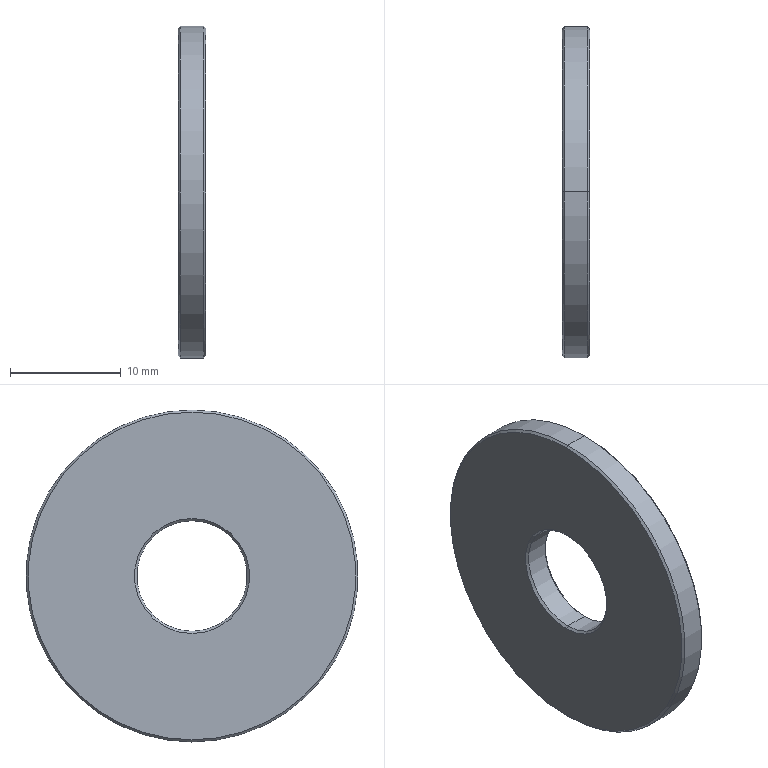Part | STEP file | WSX-SUS-M10X30-2.5-6 | 1 solid | 14 faces | box 2.5 x 30 x 30 mm | volume 1566 mm3 | cone 8 | cylinder 4 | plane 2 | commonest cylinder face diameters 10 x2 30 x2
STEP:
#1=CARTESIAN_POINT('',(0.,0.,0.));
#2=DIRECTION('',(0.,0.,1.));
#3=DIRECTION('',(1.,0.,0.));
#4=AXIS2_PLACEMENT_3D('',#1,#2,#3);
#5=CARTESIAN_POINT('',(2.5,0.,-14.8));
#6=VERTEX_POINT('',#5);
#7=CARTESIAN_POINT('',(2.5,0.,14.8));
#8=VERTEX_POINT('',#7);
#9=CARTESIAN_POINT('',(2.5,0.,0.));
#10=DIRECTION('',(1.,0.,0.));
#11=DIRECTION('',(0.,0.,1.));
#12=AXIS2_PLACEMENT_3D('',#9,#10,#11);
#13=CIRCLE('',#12,14.8);
#14=CARTESIAN_POINT('',(2.3,0.,0.));
#15=DIRECTION('',(-1.,0.,0.));
#16=DIRECTION('',(0.,0.,1.));
#17=AXIS2_PLACEMENT_3D('',#14,#15,#16);
#18=CONICAL_SURFACE('',#17,15.,0.7854);
#19=CARTESIAN_POINT('',(6.283,-0.2));
#20=DIRECTION('',(-1.,0.));
#21=VECTOR('',#20,1.);
#22=LINE('',#19,#21);
#23=(GEOMETRIC_REPRESENTATION_CONTEXT(2)PARAMETRIC_REPRESENTATION_CONTEXT()REPRESENTATION_CONTEXT('',''));
#24=DEFINITIONAL_REPRESENTATION('',(#22),#23);
#25=PCURVE('',#18,#24);
#26=CARTESIAN_POINT('',(2.5,5.,0.));
#27=DIRECTION('',(-1.,0.,0.));
#28=DIRECTION('',(0.,0.,1.));
#29=AXIS2_PLACEMENT_3D('',#26,#27,#28);
#30=PLANE('',#29);
#31=CARTESIAN_POINT('',(14.8,-5.));
#32=CARTESIAN_POINT('',(14.8,-30.634));
#33=CARTESIAN_POINT('',(-7.4,-17.817));
#34=CARTESIAN_POINT('',(-29.6,-5.));
#35=CARTESIAN_POINT('',(-7.4,7.817));
#36=CARTESIAN_POINT('',(14.8,20.634));
#37=CARTESIAN_POINT('',(14.8,-5.));
#38=(BOUNDED_CURVE()B_SPLINE_CURVE(2,(#31,#32,#33,#34,#35,#36,#37),.UNSPECIFIED.,.T.,.F.)B_SPLINE_CURVE_WITH_KNOTS((1,2,2,2,2,1),(-2.094,0.,2.094,4.189,6.283,8.378),.UNSPECIFIED.)CURVE()GEOMETRIC_REPRESENTATION_ITEM()RATIONAL_B_SPLINE_CURVE((1.,0.5,1.,0.5,1.,0.5,1.))REPRESENTATION_ITEM(''));
#39=(GEOMETRIC_REPRESENTATION_CONTEXT(2)PARAMETRIC_REPRESENTATION_CONTEXT()REPRESENTATION_CONTEXT('',''));
#40=DEFINITIONAL_REPRESENTATION('',(#38),#39);
#41=PCURVE('',#30,#40);
#42=SURFACE_CURVE('',#13,(#25,#41),.PCURVE_S1.);
#43=EDGE_CURVE('',#6,#8,#42,.T.);
#44=ORIENTED_EDGE('',*,*,#43,.F.);
#45=CARTESIAN_POINT('',(2.3,0.,-15.));
#46=VERTEX_POINT('',#45);
#47=CARTESIAN_POINT('',(2.3,0.,-15.));
#48=DIRECTION('',(-0.7071,0.,-0.7071));
#49=VECTOR('',#48,1.);
#50=LINE('',#47,#49);
#51=CARTESIAN_POINT('',(3.142,0.));
#52=DIRECTION('',(0.,1.));
#53=VECTOR('',#52,1.);
#54=LINE('',#51,#53);
#55=(GEOMETRIC_REPRESENTATION_CONTEXT(2)PARAMETRIC_REPRESENTATION_CONTEXT()REPRESENTATION_CONTEXT('',''));
#56=DEFINITIONAL_REPRESENTATION('',(#54),#55);
#57=PCURVE('',#18,#56);
#58=CARTESIAN_POINT('',(2.3,0.,0.));
#59=DIRECTION('',(-1.,0.,0.));
#60=DIRECTION('',(0.,0.,1.));
#61=AXIS2_PLACEMENT_3D('',#58,#59,#60);
#62=CONICAL_SURFACE('',#61,15.,0.7854);
#63=CARTESIAN_POINT('',(3.142,0.));
#64=DIRECTION('',(0.,1.));
#65=VECTOR('',#64,1.);
#66=LINE('',#63,#65);
#67=(GEOMETRIC_REPRESENTATION_CONTEXT(2)PARAMETRIC_REPRESENTATION_CONTEXT()REPRESENTATION_CONTEXT('',''));
#68=DEFINITIONAL_REPRESENTATION('',(#66),#67);
#69=PCURVE('',#62,#68);
#70=SURFACE_CURVE('',#50,(#57,#69),.PCURVE_S1.);
#71=EDGE_CURVE('',#6,#46,#70,.T.);
#72=ORIENTED_EDGE('',*,*,#71,.T.);
#73=CARTESIAN_POINT('',(2.3,0.,15.));
#74=VERTEX_POINT('',#73);
#75=CARTESIAN_POINT('',(2.3,0.,0.));
#76=DIRECTION('',(-1.,0.,0.));
#77=DIRECTION('',(0.,0.,1.));
#78=AXIS2_PLACEMENT_3D('',#75,#76,#77);
#79=CIRCLE('',#78,15.);
#80=CARTESIAN_POINT('',(0.,0.));
#81=DIRECTION('',(1.,0.));
#82=VECTOR('',#81,1.);
#83=LINE('',#80,#82);
#84=(GEOMETRIC_REPRESENTATION_CONTEXT(2)PARAMETRIC_REPRESENTATION_CONTEXT()REPRESENTATION_CONTEXT('',''));
#85=DEFINITIONAL_REPRESENTATION('',(#83),#84);
#86=PCURVE('',#18,#85);
#87=CARTESIAN_POINT('',(0.,0.,0.));
#88=DIRECTION('',(-1.,0.,0.));
#89=DIRECTION('',(0.,0.,1.));
#90=AXIS2_PLACEMENT_3D('',#87,#88,#89);
#91=CYLINDRICAL_SURFACE('',#90,15.);
#92=CARTESIAN_POINT('',(0.,-2.3));
#93=DIRECTION('',(1.,0.));
#94=VECTOR('',#93,1.);
#95=LINE('',#92,#94);
#96=(GEOMETRIC_REPRESENTATION_CONTEXT(2)PARAMETRIC_REPRESENTATION_CONTEXT()REPRESENTATION_CONTEXT('',''));
#97=DEFINITIONAL_REPRESENTATION('',(#95),#96);
#98=PCURVE('',#91,#97);
#99=SURFACE_CURVE('',#79,(#86,#98),.PCURVE_S1.);
#100=EDGE_CURVE('',#74,#46,#99,.T.);
#101=ORIENTED_EDGE('',*,*,#100,.F.);
#102=CARTESIAN_POINT('',(2.3,0.,15.));
#103=DIRECTION('',(-0.7071,0.,0.7071));
#104=VECTOR('',#103,1.);
#105=LINE('',#102,#104);
#106=CARTESIAN_POINT('',(0.,0.));
#107=DIRECTION('',(0.,1.));
#108=VECTOR('',#107,1.);
#109=LINE('',#106,#108);
#110=(GEOMETRIC_REPRESENTATION_CONTEXT(2)PARAMETRIC_REPRESENTATION_CONTEXT()REPRESENTATION_CONTEXT('',''));
#111=DEFINITIONAL_REPRESENTATION('',(#109),#110);
#112=PCURVE('',#18,#111);
#113=CARTESIAN_POINT('',(6.283,0.));
#114=DIRECTION('',(0.,1.));
#115=VECTOR('',#114,1.);
#116=LINE('',#113,#115);
#117=(GEOMETRIC_REPRESENTATION_CONTEXT(2)PARAMETRIC_REPRESENTATION_CONTEXT()REPRESENTATION_CONTEXT('',''));
#118=DEFINITIONAL_REPRESENTATION('',(#116),#117);
#119=PCURVE('',#62,#118);
#120=SURFACE_CURVE('',#105,(#112,#119),.PCURVE_S1.);
#121=EDGE_CURVE('',#8,#74,#120,.T.);
#122=ORIENTED_EDGE('',*,*,#121,.F.);
#123=EDGE_LOOP('',(#44,#72,#101,#122));
#124=FACE_BOUND('',#123,.T.);
#125=ADVANCED_FACE('',(#124),#18,.T.);
#126=CARTESIAN_POINT('',(2.3,0.,-5.));
#127=VERTEX_POINT('',#126);
#128=CARTESIAN_POINT('',(2.5,0.,-5.2));
#129=VERTEX_POINT('',#128);
#130=CARTESIAN_POINT('',(2.5,0.,-5.2));
#131=DIRECTION('',(0.7071,0.,-0.7071));
#132=VECTOR('',#131,1.);
#133=LINE('',#130,#132);
#134=CARTESIAN_POINT('',(2.5,0.,0.));
#135=DIRECTION('',(1.,0.,0.));
#136=DIRECTION('',(0.,0.,-1.));
#137=AXIS2_PLACEMENT_3D('',#134,#135,#136);
#138=CONICAL_SURFACE('',#137,5.2,0.7854);
#139=CARTESIAN_POINT('',(6.283,0.));
#140=DIRECTION('',(0.,1.));
#141=VECTOR('',#140,1.);
#142=LINE('',#139,#141);
#143=(GEOMETRIC_REPRESENTATION_CONTEXT(2)PARAMETRIC_REPRESENTATION_CONTEXT()REPRESENTATION_CONTEXT('',''));
#144=DEFINITIONAL_REPRESENTATION('',(#142),#143);
#145=PCURVE('',#138,#144);
#146=CARTESIAN_POINT('',(2.5,0.,0.));
#147=DIRECTION('',(1.,0.,0.));
#148=DIRECTION('',(0.,0.,-1.));
#149=AXIS2_PLACEMENT_3D('',#146,#147,#148);
#150=CONICAL_SURFACE('',#149,5.2,0.7854);
#151=CARTESIAN_POINT('',(0.,0.));
#152=DIRECTION('',(0.,1.));
#153=VECTOR('',#152,1.);
#154=LINE('',#151,#153);
#155=(GEOMETRIC_REPRESENTATION_CONTEXT(2)PARAMETRIC_REPRESENTATION_CONTEXT()REPRESENTATION_CONTEXT('',''));
#156=DEFINITIONAL_REPRESENTATION('',(#154),#155);
#157=PCURVE('',#150,#156);
#158=SURFACE_CURVE('',#133,(#145,#157),.PCURVE_S1.);
#159=EDGE_CURVE('',#127,#129,#158,.T.);
#160=ORIENTED_EDGE('',*,*,#159,.T.);
#161=CARTESIAN_POINT('',(2.5,0.,5.2));
#162=VERTEX_POINT('',#161);
#163=CARTESIAN_POINT('',(2.5,0.,0.));
#164=DIRECTION('',(-1.,0.,0.));
#165=DIRECTION('',(0.,0.,1.));
#166=AXIS2_PLACEMENT_3D('',#163,#164,#165);
#167=CIRCLE('',#166,5.2);
#168=CARTESIAN_POINT('',(9.425,0.));
#169=DIRECTION('',(-1.,0.));
#170=VECTOR('',#169,1.);
#171=LINE('',#168,#170);
#172=(GEOMETRIC_REPRESENTATION_CONTEXT(2)PARAMETRIC_REPRESENTATION_CONTEXT()REPRESENTATION_CONTEXT('',''));
#173=DEFINITIONAL_REPRESENTATION('',(#171),#172);
#174=PCURVE('',#138,#173);
#175=CARTESIAN_POINT('',(0.,-5.));
#176=DIRECTION('',(1.,0.));
#177=AXIS2_PLACEMENT_2D('',#175,#176);
#178=CIRCLE('',#177,5.2);
#179=(GEOMETRIC_REPRESENTATION_CONTEXT(2)PARAMETRIC_REPRESENTATION_CONTEXT()REPRESENTATION_CONTEXT('',''));
#180=DEFINITIONAL_REPRESENTATION('',(#178),#179);
#181=PCURVE('',#30,#180);
#182=SURFACE_CURVE('',#167,(#174,#181),.PCURVE_S1.);
#183=EDGE_CURVE('',#129,#162,#182,.T.);
#184=ORIENTED_EDGE('',*,*,#183,.T.);
#185=CARTESIAN_POINT('',(2.3,0.,5.));
#186=VERTEX_POINT('',#185);
#187=CARTESIAN_POINT('',(2.5,0.,5.2));
#188=DIRECTION('',(0.7071,0.,0.7071));
#189=VECTOR('',#188,1.);
#190=LINE('',#187,#189);
#191=CARTESIAN_POINT('',(3.142,0.));
#192=DIRECTION('',(0.,1.));
#193=VECTOR('',#192,1.);
#194=LINE('',#191,#193);
#195=(GEOMETRIC_REPRESENTATION_CONTEXT(2)PARAMETRIC_REPRESENTATION_CONTEXT()REPRESENTATION_CONTEXT('',''));
#196=DEFINITIONAL_REPRESENTATION('',(#194),#195);
#197=PCURVE('',#138,#196);
#198=CARTESIAN_POINT('',(3.142,0.));
#199=DIRECTION('',(0.,1.));
#200=VECTOR('',#199,1.);
#201=LINE('',#198,#200);
#202=(GEOMETRIC_REPRESENTATION_CONTEXT(2)PARAMETRIC_REPRESENTATION_CONTEXT()REPRESENTATION_CONTEXT('',''));
#203=DEFINITIONAL_REPRESENTATION('',(#201),#202);
#204=PCURVE('',#150,#203);
#205=SURFACE_CURVE('',#190,(#197,#204),.PCURVE_S1.);
#206=EDGE_CURVE('',#186,#162,#205,.T.);
#207=ORIENTED_EDGE('',*,*,#206,.F.);
#208=CARTESIAN_POINT('',(2.3,0.,0.));
#209=DIRECTION('',(1.,0.,0.));
#210=DIRECTION('',(0.,0.,1.));
#211=AXIS2_PLACEMENT_3D('',#208,#209,#210);
#212=CIRCLE('',#211,5.);
#213=CARTESIAN_POINT('',(3.142,-0.2));
#214=DIRECTION('',(1.,0.));
#215=VECTOR('',#214,1.);
#216=LINE('',#213,#215);
#217=(GEOMETRIC_REPRESENTATION_CONTEXT(2)PARAMETRIC_REPRESENTATION_CONTEXT()REPRESENTATION_CONTEXT('',''));
#218=DEFINITIONAL_REPRESENTATION('',(#216),#217);
#219=PCURVE('',#138,#218);
#220=CARTESIAN_POINT('',(0.,0.,0.));
#221=DIRECTION('',(-1.,0.,0.));
#222=DIRECTION('',(0.,0.,1.));
#223=AXIS2_PLACEMENT_3D('',#220,#221,#222);
#224=CYLINDRICAL_SURFACE('',#223,5.);
#225=CARTESIAN_POINT('',(6.283,-2.3));
#226=DIRECTION('',(-1.,0.));
#227=VECTOR('',#226,1.);
#228=LINE('',#225,#227);
#229=(GEOMETRIC_REPRESENTATION_CONTEXT(2)PARAMETRIC_REPRESENTATION_CONTEXT()REPRESENTATION_CONTEXT('',''));
#230=DEFINITIONAL_REPRESENTATION('',(#228),#229);
#231=PCURVE('',#224,#230);
#232=SURFACE_CURVE('',#212,(#219,#231),.PCURVE_S1.);
#233=EDGE_CURVE('',#186,#127,#232,.T.);
#234=ORIENTED_EDGE('',*,*,#233,.T.);
#235=EDGE_LOOP('',(#160,#184,#207,#234));
#236=FACE_BOUND('',#235,.F.);
#237=ADVANCED_FACE('',(#236),#138,.F.);
#238=CARTESIAN_POINT('',(0.,0.,14.8));
#239=VERTEX_POINT('',#238);
#240=CARTESIAN_POINT('',(0.,0.,-14.8));
#241=VERTEX_POINT('',#240);
#242=CARTESIAN_POINT('',(0.,0.,0.));
#243=DIRECTION('',(-1.,0.,0.));
#244=DIRECTION('',(0.,0.,-1.));
#245=AXIS2_PLACEMENT_3D('',#242,#243,#244);
#246=CIRCLE('',#245,14.8);
#247=CARTESIAN_POINT('',(0.,0.,0.));
#248=DIRECTION('',(1.,0.,0.));
#249=DIRECTION('',(0.,0.,-1.));
#250=AXIS2_PLACEMENT_3D('',#247,#248,#249);
#251=CONICAL_SURFACE('',#250,14.8,0.7854);
#252=CARTESIAN_POINT('',(6.283,0.));
#253=DIRECTION('',(-1.,0.));
#254=VECTOR('',#253,1.);
#255=LINE('',#252,#254);
#256=(GEOMETRIC_REPRESENTATION_CONTEXT(2)PARAMETRIC_REPRESENTATION_CONTEXT()REPRESENTATION_CONTEXT('',''));
#257=DEFINITIONAL_REPRESENTATION('',(#255),#256);
#258=PCURVE('',#251,#257);
#259=CARTESIAN_POINT('',(0.,5.,0.));
#260=DIRECTION('',(1.,0.,0.));
#261=DIRECTION('',(0.,0.,-1.));
#262=AXIS2_PLACEMENT_3D('',#259,#260,#261);
#263=PLANE('',#262);
#264=CARTESIAN_POINT('',(14.8,-5.));
#265=CARTESIAN_POINT('',(14.8,-30.634));
#266=CARTESIAN_POINT('',(-7.4,-17.817));
#267=CARTESIAN_POINT('',(-29.6,-5.));
#268=CARTESIAN_POINT('',(-7.4,7.817));
#269=CARTESIAN_POINT('',(14.8,20.634));
#270=CARTESIAN_POINT('',(14.8,-5.));
#271=(BOUNDED_CURVE()B_SPLINE_CURVE(2,(#264,#265,#266,#267,#268,#269,#270),.UNSPECIFIED.,.T.,.F.)B_SPLINE_CURVE_WITH_KNOTS((1,2,2,2,2,1),(-2.094,0.,2.094,4.189,6.283,8.378),.UNSPECIFIED.)CURVE()GEOMETRIC_REPRESENTATION_ITEM()RATIONAL_B_SPLINE_CURVE((1.,0.5,1.,0.5,1.,0.5,1.))REPRESENTATION_ITEM(''));
#272=(GEOMETRIC_REPRESENTATION_CONTEXT(2)PARAMETRIC_REPRESENTATION_CONTEXT()REPRESENTATION_CONTEXT('',''));
#273=DEFINITIONAL_REPRESENTATION('',(#271),#272);
#274=PCURVE('',#263,#273);
#275=SURFACE_CURVE('',#246,(#258,#274),.PCURVE_S1.);
#276=EDGE_CURVE('',#239,#241,#275,.T.);
#277=ORIENTED_EDGE('',*,*,#276,.F.);
#278=CARTESIAN_POINT('',(0.2,0.,15.));
#279=VERTEX_POINT('',#278);
#280=CARTESIAN_POINT('',(0.,0.,14.8));
#281=DIRECTION('',(0.7071,0.,0.7071));
#282=VECTOR('',#281,1.);
#283=LINE('',#280,#282);
#284=CARTESIAN_POINT('',(3.142,0.));
#285=DIRECTION('',(0.,1.));
#286=VECTOR('',#285,1.);
#287=LINE('',#284,#286);
#288=(GEOMETRIC_REPRESENTATION_CONTEXT(2)PARAMETRIC_REPRESENTATION_CONTEXT()REPRESENTATION_CONTEXT('',''));
#289=DEFINITIONAL_REPRESENTATION('',(#287),#288);
#290=PCURVE('',#251,#289);
#291=CARTESIAN_POINT('',(0.,0.,0.));
#292=DIRECTION('',(1.,0.,0.));
#293=DIRECTION('',(0.,0.,-1.));
#294=AXIS2_PLACEMENT_3D('',#291,#292,#293);
#295=CONICAL_SURFACE('',#294,14.8,0.7854);
#296=CARTESIAN_POINT('',(3.142,0.));
#297=DIRECTION('',(0.,1.));
#298=VECTOR('',#297,1.);
#299=LINE('',#296,#298);
#300=(GEOMETRIC_REPRESENTATION_CONTEXT(2)PARAMETRIC_REPRESENTATION_CONTEXT()REPRESENTATION_CONTEXT('',''));
#301=DEFINITIONAL_REPRESENTATION('',(#299),#300);
#302=PCURVE('',#295,#301);
#303=SURFACE_CURVE('',#283,(#290,#302),.PCURVE_S1.);
#304=EDGE_CURVE('',#239,#279,#303,.T.);
#305=ORIENTED_EDGE('',*,*,#304,.T.);
#306=CARTESIAN_POINT('',(0.2,0.,-15.));
#307=VERTEX_POINT('',#306);
#308=CARTESIAN_POINT('',(0.2,0.,0.));
#309=DIRECTION('',(1.,0.,0.));
#310=DIRECTION('',(0.,0.,-1.));
#311=AXIS2_PLACEMENT_3D('',#308,#309,#310);
#312=CIRCLE('',#311,15.);
#313=CARTESIAN_POINT('',(0.,0.2));
#314=DIRECTION('',(1.,0.));
#315=VECTOR('',#314,1.);
#316=LINE('',#313,#315);
#317=(GEOMETRIC_REPRESENTATION_CONTEXT(2)PARAMETRIC_REPRESENTATION_CONTEXT()REPRESENTATION_CONTEXT('',''));
#318=DEFINITIONAL_REPRESENTATION('',(#316),#317);
#319=PCURVE('',#251,#318);
#320=CARTESIAN_POINT('',(3.142,-0.2));
#321=DIRECTION('',(-1.,0.));
#322=VECTOR('',#321,1.);
#323=LINE('',#320,#322);
#324=(GEOMETRIC_REPRESENTATION_CONTEXT(2)PARAMETRIC_REPRESENTATION_CONTEXT()REPRESENTATION_CONTEXT('',''));
#325=DEFINITIONAL_REPRESENTATION('',(#323),#324);
#326=PCURVE('',#91,#325);
#327=SURFACE_CURVE('',#312,(#319,#326),.PCURVE_S1.);
#328=EDGE_CURVE('',#307,#279,#327,.T.);
#329=ORIENTED_EDGE('',*,*,#328,.F.);
#330=CARTESIAN_POINT('',(0.,0.,-14.8));
#331=DIRECTION('',(0.7071,0.,-0.7071));
#332=VECTOR('',#331,1.);
#333=LINE('',#330,#332);
#334=CARTESIAN_POINT('',(0.,0.));
#335=DIRECTION('',(0.,1.));
#336=VECTOR('',#335,1.);
#337=LINE('',#334,#336);
#338=(GEOMETRIC_REPRESENTATION_CONTEXT(2)PARAMETRIC_REPRESENTATION_CONTEXT()REPRESENTATION_CONTEXT('',''));
#339=DEFINITIONAL_REPRESENTATION('',(#337),#338);
#340=PCURVE('',#251,#339);
#341=CARTESIAN_POINT('',(6.283,0.));
#342=DIRECTION('',(0.,1.));
#343=VECTOR('',#342,1.);
#344=LINE('',#341,#343);
#345=(GEOMETRIC_REPRESENTATION_CONTEXT(2)PARAMETRIC_REPRESENTATION_CONTEXT()REPRESENTATION_CONTEXT('',''));
#346=DEFINITIONAL_REPRESENTATION('',(#344),#345);
#347=PCURVE('',#295,#346);
#348=SURFACE_CURVE('',#333,(#340,#347),.PCURVE_S1.);
#349=EDGE_CURVE('',#241,#307,#348,.T.);
#350=ORIENTED_EDGE('',*,*,#349,.F.);
#351=EDGE_LOOP('',(#277,#305,#329,#350));
#352=FACE_BOUND('',#351,.T.);
#353=ADVANCED_FACE('',(#352),#251,.T.);
#354=CARTESIAN_POINT('',(0.2,0.,5.));
#355=VERTEX_POINT('',#354);
#356=CARTESIAN_POINT('',(0.,0.,5.2));
#357=VERTEX_POINT('',#356);
#358=CARTESIAN_POINT('',(0.2,0.,5.));
#359=DIRECTION('',(-0.7071,0.,0.7071));
#360=VECTOR('',#359,1.);
#361=LINE('',#358,#360);
#362=CARTESIAN_POINT('',(0.2,0.,0.));
#363=DIRECTION('',(-1.,0.,0.));
#364=DIRECTION('',(0.,0.,1.));
#365=AXIS2_PLACEMENT_3D('',#362,#363,#364);
#366=CONICAL_SURFACE('',#365,5.,0.7854);
#367=CARTESIAN_POINT('',(6.283,0.));
#368=DIRECTION('',(0.,1.));
#369=VECTOR('',#368,1.);
#370=LINE('',#367,#369);
#371=(GEOMETRIC_REPRESENTATION_CONTEXT(2)PARAMETRIC_REPRESENTATION_CONTEXT()REPRESENTATION_CONTEXT('',''));
#372=DEFINITIONAL_REPRESENTATION('',(#370),#371);
#373=PCURVE('',#366,#372);
#374=CARTESIAN_POINT('',(0.2,0.,0.));
#375=DIRECTION('',(-1.,0.,0.));
#376=DIRECTION('',(0.,0.,1.));
#377=AXIS2_PLACEMENT_3D('',#374,#375,#376);
#378=CONICAL_SURFACE('',#377,5.,0.7854);
#379=CARTESIAN_POINT('',(0.,0.));
#380=DIRECTION('',(0.,1.));
#381=VECTOR('',#380,1.);
#382=LINE('',#379,#381);
#383=(GEOMETRIC_REPRESENTATION_CONTEXT(2)PARAMETRIC_REPRESENTATION_CONTEXT()REPRESENTATION_CONTEXT('',''));
#384=DEFINITIONAL_REPRESENTATION('',(#382),#383);
#385=PCURVE('',#378,#384);
#386=SURFACE_CURVE('',#361,(#373,#385),.PCURVE_S1.);
#387=EDGE_CURVE('',#355,#357,#386,.T.);
#388=ORIENTED_EDGE('',*,*,#387,.T.);
#389=CARTESIAN_POINT('',(0.,0.,-5.2));
#390=VERTEX_POINT('',#389);
#391=CARTESIAN_POINT('',(0.,0.,0.));
#392=DIRECTION('',(1.,0.,0.));
#393=DIRECTION('',(0.,0.,-1.));
#394=AXIS2_PLACEMENT_3D('',#391,#392,#393);
#395=CIRCLE('',#394,5.2);
#396=CARTESIAN_POINT('',(9.425,0.2));
#397=DIRECTION('',(-1.,0.));
#398=VECTOR('',#397,1.);
#399=LINE('',#396,#398);
#400=(GEOMETRIC_REPRESENTATION_CONTEXT(2)PARAMETRIC_REPRESENTATION_CONTEXT()REPRESENTATION_CONTEXT('',''));
#401=DEFINITIONAL_REPRESENTATION('',(#399),#400);
#402=PCURVE('',#366,#401);
#403=CARTESIAN_POINT('',(0.,-5.));
#404=DIRECTION('',(1.,0.));
#405=AXIS2_PLACEMENT_2D('',#403,#404);
#406=CIRCLE('',#405,5.2);
#407=(GEOMETRIC_REPRESENTATION_CONTEXT(2)PARAMETRIC_REPRESENTATION_CONTEXT()REPRESENTATION_CONTEXT('',''));
#408=DEFINITIONAL_REPRESENTATION('',(#406),#407);
#409=PCURVE('',#263,#408);
#410=SURFACE_CURVE('',#395,(#402,#409),.PCURVE_S1.);
#411=EDGE_CURVE('',#357,#390,#410,.T.);
#412=ORIENTED_EDGE('',*,*,#411,.T.);
#413=CARTESIAN_POINT('',(0.2,0.,-5.));
#414=VERTEX_POINT('',#413);
#415=CARTESIAN_POINT('',(0.2,0.,-5.));
#416=DIRECTION('',(-0.7071,0.,-0.7071));
#417=VECTOR('',#416,1.);
#418=LINE('',#415,#417);
#419=CARTESIAN_POINT('',(3.142,0.));
#420=DIRECTION('',(0.,1.));
#421=VECTOR('',#420,1.);
#422=LINE('',#419,#421);
#423=(GEOMETRIC_REPRESENTATION_CONTEXT(2)PARAMETRIC_REPRESENTATION_CONTEXT()REPRESENTATION_CONTEXT('',''));
#424=DEFINITIONAL_REPRESENTATION('',(#422),#423);
#425=PCURVE('',#366,#424);
#426=CARTESIAN_POINT('',(3.142,0.));
#427=DIRECTION('',(0.,1.));
#428=VECTOR('',#427,1.);
#429=LINE('',#426,#428);
#430=(GEOMETRIC_REPRESENTATION_CONTEXT(2)PARAMETRIC_REPRESENTATION_CONTEXT()REPRESENTATION_CONTEXT('',''));
#431=DEFINITIONAL_REPRESENTATION('',(#429),#430);
#432=PCURVE('',#378,#431);
#433=SURFACE_CURVE('',#418,(#425,#432),.PCURVE_S1.);
#434=EDGE_CURVE('',#414,#390,#433,.T.);
#435=ORIENTED_EDGE('',*,*,#434,.F.);
#436=CARTESIAN_POINT('',(0.2,0.,0.));
#437=DIRECTION('',(-1.,0.,0.));
#438=DIRECTION('',(0.,0.,-1.));
#439=AXIS2_PLACEMENT_3D('',#436,#437,#438);
#440=CIRCLE('',#439,5.);
#441=CARTESIAN_POINT('',(3.142,0.));
#442=DIRECTION('',(1.,0.));
#443=VECTOR('',#442,1.);
#444=LINE('',#441,#443);
#445=(GEOMETRIC_REPRESENTATION_CONTEXT(2)PARAMETRIC_REPRESENTATION_CONTEXT()REPRESENTATION_CONTEXT('',''));
#446=DEFINITIONAL_REPRESENTATION('',(#444),#445);
#447=PCURVE('',#366,#446);
#448=CARTESIAN_POINT('',(3.142,-0.2));
#449=DIRECTION('',(1.,0.));
#450=VECTOR('',#449,1.);
#451=LINE('',#448,#450);
#452=(GEOMETRIC_REPRESENTATION_CONTEXT(2)PARAMETRIC_REPRESENTATION_CONTEXT()REPRESENTATION_CONTEXT('',''));
#453=DEFINITIONAL_REPRESENTATION('',(#451),#452);
#454=PCURVE('',#224,#453);
#455=SURFACE_CURVE('',#440,(#447,#454),.PCURVE_S1.);
#456=EDGE_CURVE('',#414,#355,#455,.T.);
#457=ORIENTED_EDGE('',*,*,#456,.T.);
#458=EDGE_LOOP('',(#388,#412,#435,#457));
#459=FACE_BOUND('',#458,.F.);
#460=ADVANCED_FACE('',(#459),#366,.F.);
#461=CARTESIAN_POINT('',(0.,0.,5.));
#462=DIRECTION('',(-1.,0.,0.));
#463=VECTOR('',#462,1.);
#464=LINE('',#461,#463);
#465=CARTESIAN_POINT('',(6.283,0.));
#466=DIRECTION('',(0.,1.));
#467=VECTOR('',#466,1.);
#468=LINE('',#465,#467);
#469=(GEOMETRIC_REPRESENTATION_CONTEXT(2)PARAMETRIC_REPRESENTATION_CONTEXT()REPRESENTATION_CONTEXT('',''));
#470=DEFINITIONAL_REPRESENTATION('',(#468),#469);
#471=PCURVE('',#224,#470);
#472=CARTESIAN_POINT('',(0.,0.,0.));
#473=DIRECTION('',(-1.,0.,0.));
#474=DIRECTION('',(0.,0.,1.));
#475=AXIS2_PLACEMENT_3D('',#472,#473,#474);
#476=CYLINDRICAL_SURFACE('',#475,5.);
#477=CARTESIAN_POINT('',(0.,0.));
#478=DIRECTION('',(0.,1.));
#479=VECTOR('',#478,1.);
#480=LINE('',#477,#479);
#481=(GEOMETRIC_REPRESENTATION_CONTEXT(2)PARAMETRIC_REPRESENTATION_CONTEXT()REPRESENTATION_CONTEXT('',''));
#482=DEFINITIONAL_REPRESENTATION('',(#480),#481);
#483=PCURVE('',#476,#482);
#484=SURFACE_CURVE('',#464,(#471,#483),.PCURVE_S1.);
#485=EDGE_CURVE('',#186,#355,#484,.T.);
#486=ORIENTED_EDGE('',*,*,#485,.T.);
#487=ORIENTED_EDGE('',*,*,#456,.F.);
#488=CARTESIAN_POINT('',(0.,0.,-5.));
#489=DIRECTION('',(-1.,0.,0.));
#490=VECTOR('',#489,1.);
#491=LINE('',#488,#490);
#492=CARTESIAN_POINT('',(3.142,0.));
#493=DIRECTION('',(0.,1.));
#494=VECTOR('',#493,1.);
#495=LINE('',#492,#494);
#496=(GEOMETRIC_REPRESENTATION_CONTEXT(2)PARAMETRIC_REPRESENTATION_CONTEXT()REPRESENTATION_CONTEXT('',''));
#497=DEFINITIONAL_REPRESENTATION('',(#495),#496);
#498=PCURVE('',#224,#497);
#499=CARTESIAN_POINT('',(3.142,0.));
#500=DIRECTION('',(0.,1.));
#501=VECTOR('',#500,1.);
#502=LINE('',#499,#501);
#503=(GEOMETRIC_REPRESENTATION_CONTEXT(2)PARAMETRIC_REPRESENTATION_CONTEXT()REPRESENTATION_CONTEXT('',''));
#504=DEFINITIONAL_REPRESENTATION('',(#502),#503);
#505=PCURVE('',#476,#504);
#506=SURFACE_CURVE('',#491,(#498,#505),.PCURVE_S1.);
#507=EDGE_CURVE('',#127,#414,#506,.T.);
#508=ORIENTED_EDGE('',*,*,#507,.F.);
#509=ORIENTED_EDGE('',*,*,#233,.F.);
#510=EDGE_LOOP('',(#486,#487,#508,#509));
#511=FACE_BOUND('',#510,.F.);
#512=ADVANCED_FACE('',(#511),#224,.F.);
#513=ORIENTED_EDGE('',*,*,#100,.T.);
#514=CARTESIAN_POINT('',(0.,0.,-15.));
#515=DIRECTION('',(-1.,0.,0.));
#516=VECTOR('',#515,1.);
#517=LINE('',#514,#516);
#518=CARTESIAN_POINT('',(3.142,0.));
#519=DIRECTION('',(0.,1.));
#520=VECTOR('',#519,1.);
#521=LINE('',#518,#520);
#522=(GEOMETRIC_REPRESENTATION_CONTEXT(2)PARAMETRIC_REPRESENTATION_CONTEXT()REPRESENTATION_CONTEXT('',''));
#523=DEFINITIONAL_REPRESENTATION('',(#521),#522);
#524=PCURVE('',#91,#523);
#525=CARTESIAN_POINT('',(0.,0.,0.));
#526=DIRECTION('',(-1.,0.,0.));
#527=DIRECTION('',(0.,0.,1.));
#528=AXIS2_PLACEMENT_3D('',#525,#526,#527);
#529=CYLINDRICAL_SURFACE('',#528,15.);
#530=CARTESIAN_POINT('',(3.142,0.));
#531=DIRECTION('',(0.,1.));
#532=VECTOR('',#531,1.);
#533=LINE('',#530,#532);
#534=(GEOMETRIC_REPRESENTATION_CONTEXT(2)PARAMETRIC_REPRESENTATION_CONTEXT()REPRESENTATION_CONTEXT('',''));
#535=DEFINITIONAL_REPRESENTATION('',(#533),#534);
#536=PCURVE('',#529,#535);
#537=SURFACE_CURVE('',#517,(#524,#536),.PCURVE_S1.);
#538=EDGE_CURVE('',#46,#307,#537,.T.);
#539=ORIENTED_EDGE('',*,*,#538,.T.);
#540=ORIENTED_EDGE('',*,*,#328,.T.);
#541=CARTESIAN_POINT('',(0.,0.,15.));
#542=DIRECTION('',(-1.,0.,0.));
#543=VECTOR('',#542,1.);
#544=LINE('',#541,#543);
#545=CARTESIAN_POINT('',(0.,0.));
#546=DIRECTION('',(0.,1.));
#547=VECTOR('',#546,1.);
#548=LINE('',#545,#547);
#549=(GEOMETRIC_REPRESENTATION_CONTEXT(2)PARAMETRIC_REPRESENTATION_CONTEXT()REPRESENTATION_CONTEXT('',''));
#550=DEFINITIONAL_REPRESENTATION('',(#548),#549);
#551=PCURVE('',#91,#550);
#552=CARTESIAN_POINT('',(6.283,0.));
#553=DIRECTION('',(0.,1.));
#554=VECTOR('',#553,1.);
#555=LINE('',#552,#554);
#556=(GEOMETRIC_REPRESENTATION_CONTEXT(2)PARAMETRIC_REPRESENTATION_CONTEXT()REPRESENTATION_CONTEXT('',''));
#557=DEFINITIONAL_REPRESENTATION('',(#555),#556);
#558=PCURVE('',#529,#557);
#559=SURFACE_CURVE('',#544,(#551,#558),.PCURVE_S1.);
#560=EDGE_CURVE('',#74,#279,#559,.T.);
#561=ORIENTED_EDGE('',*,*,#560,.F.);
#562=EDGE_LOOP('',(#513,#539,#540,#561));
#563=FACE_BOUND('',#562,.T.);
#564=ADVANCED_FACE('',(#563),#91,.T.);
#565=ORIENTED_EDGE('',*,*,#411,.T.);
#566=CARTESIAN_POINT('',(0.,0.,0.));
#567=DIRECTION('',(1.,0.,0.));
#568=DIRECTION('',(0.,0.,-1.));
#569=AXIS2_PLACEMENT_3D('',#566,#567,#568);
#570=CIRCLE('',#569,5.2);
#571=CARTESIAN_POINT('',(0.,-5.));
#572=DIRECTION('',(1.,0.));
#573=AXIS2_PLACEMENT_2D('',#571,#572);
#574=CIRCLE('',#573,5.2);
#575=(GEOMETRIC_REPRESENTATION_CONTEXT(2)PARAMETRIC_REPRESENTATION_CONTEXT()REPRESENTATION_CONTEXT('',''));
#576=DEFINITIONAL_REPRESENTATION('',(#574),#575);
#577=PCURVE('',#263,#576);
#578=CARTESIAN_POINT('',(3.142,0.2));
#579=DIRECTION('',(-1.,0.));
#580=VECTOR('',#579,1.);
#581=LINE('',#578,#580);
#582=(GEOMETRIC_REPRESENTATION_CONTEXT(2)PARAMETRIC_REPRESENTATION_CONTEXT()REPRESENTATION_CONTEXT('',''));
#583=DEFINITIONAL_REPRESENTATION('',(#581),#582);
#584=PCURVE('',#378,#583);
#585=SURFACE_CURVE('',#570,(#577,#584),.PCURVE_S1.);
#586=EDGE_CURVE('',#390,#357,#585,.T.);
#587=ORIENTED_EDGE('',*,*,#586,.T.);
#588=EDGE_LOOP('',(#565,#587));
#589=FACE_BOUND('',#588,.T.);
#590=CARTESIAN_POINT('',(0.,0.,0.));
#591=DIRECTION('',(-1.,0.,0.));
#592=DIRECTION('',(0.,0.,-1.));
#593=AXIS2_PLACEMENT_3D('',#590,#591,#592);
#594=CIRCLE('',#593,14.8);
#595=CARTESIAN_POINT('',(14.8,-5.));
#596=CARTESIAN_POINT('',(14.8,-30.634));
#597=CARTESIAN_POINT('',(-7.4,-17.817));
#598=CARTESIAN_POINT('',(-29.6,-5.));
#599=CARTESIAN_POINT('',(-7.4,7.817));
#600=CARTESIAN_POINT('',(14.8,20.634));
#601=CARTESIAN_POINT('',(14.8,-5.));
#602=(BOUNDED_CURVE()B_SPLINE_CURVE(2,(#595,#596,#597,#598,#599,#600,#601),.UNSPECIFIED.,.T.,.F.)B_SPLINE_CURVE_WITH_KNOTS((1,2,2,2,2,1),(-2.094,0.,2.094,4.189,6.283,8.378),.UNSPECIFIED.)CURVE()GEOMETRIC_REPRESENTATION_ITEM()RATIONAL_B_SPLINE_CURVE((1.,0.5,1.,0.5,1.,0.5,1.))REPRESENTATION_ITEM(''));
#603=(GEOMETRIC_REPRESENTATION_CONTEXT(2)PARAMETRIC_REPRESENTATION_CONTEXT()REPRESENTATION_CONTEXT('',''));
#604=DEFINITIONAL_REPRESENTATION('',(#602),#603);
#605=PCURVE('',#263,#604);
#606=CARTESIAN_POINT('',(6.283,0.));
#607=DIRECTION('',(-1.,0.));
#608=VECTOR('',#607,1.);
#609=LINE('',#606,#608);
#610=(GEOMETRIC_REPRESENTATION_CONTEXT(2)PARAMETRIC_REPRESENTATION_CONTEXT()REPRESENTATION_CONTEXT('',''));
#611=DEFINITIONAL_REPRESENTATION('',(#609),#610);
#612=PCURVE('',#295,#611);
#613=SURFACE_CURVE('',#594,(#605,#612),.PCURVE_S1.);
#614=EDGE_CURVE('',#241,#239,#613,.T.);
#615=ORIENTED_EDGE('',*,*,#614,.T.);
#616=ORIENTED_EDGE('',*,*,#276,.T.);
#617=EDGE_LOOP('',(#615,#616));
#618=FACE_BOUND('',#617,.T.);
#619=ADVANCED_FACE('',(#589,#618),#263,.F.);
#620=ORIENTED_EDGE('',*,*,#538,.F.);
#621=CARTESIAN_POINT('',(2.3,0.,0.));
#622=DIRECTION('',(-1.,0.,0.));
#623=DIRECTION('',(0.,0.,1.));
#624=AXIS2_PLACEMENT_3D('',#621,#622,#623);
#625=CIRCLE('',#624,15.);
#626=CARTESIAN_POINT('',(0.,-2.3));
#627=DIRECTION('',(1.,0.));
#628=VECTOR('',#627,1.);
#629=LINE('',#626,#628);
#630=(GEOMETRIC_REPRESENTATION_CONTEXT(2)PARAMETRIC_REPRESENTATION_CONTEXT()REPRESENTATION_CONTEXT('',''));
#631=DEFINITIONAL_REPRESENTATION('',(#629),#630);
#632=PCURVE('',#529,#631);
#633=CARTESIAN_POINT('',(0.,0.));
#634=DIRECTION('',(1.,0.));
#635=VECTOR('',#634,1.);
#636=LINE('',#633,#635);
#637=(GEOMETRIC_REPRESENTATION_CONTEXT(2)PARAMETRIC_REPRESENTATION_CONTEXT()REPRESENTATION_CONTEXT('',''));
#638=DEFINITIONAL_REPRESENTATION('',(#636),#637);
#639=PCURVE('',#62,#638);
#640=SURFACE_CURVE('',#625,(#632,#639),.PCURVE_S1.);
#641=EDGE_CURVE('',#46,#74,#640,.T.);
#642=ORIENTED_EDGE('',*,*,#641,.T.);
#643=ORIENTED_EDGE('',*,*,#560,.T.);
#644=CARTESIAN_POINT('',(0.2,0.,0.));
#645=DIRECTION('',(1.,0.,0.));
#646=DIRECTION('',(0.,0.,-1.));
#647=AXIS2_PLACEMENT_3D('',#644,#645,#646);
#648=CIRCLE('',#647,15.);
#649=CARTESIAN_POINT('',(9.425,-0.2));
#650=DIRECTION('',(-1.,0.));
#651=VECTOR('',#650,1.);
#652=LINE('',#649,#651);
#653=(GEOMETRIC_REPRESENTATION_CONTEXT(2)PARAMETRIC_REPRESENTATION_CONTEXT()REPRESENTATION_CONTEXT('',''));
#654=DEFINITIONAL_REPRESENTATION('',(#652),#653);
#655=PCURVE('',#529,#654);
#656=CARTESIAN_POINT('',(0.,0.2));
#657=DIRECTION('',(1.,0.));
#658=VECTOR('',#657,1.);
#659=LINE('',#656,#658);
#660=(GEOMETRIC_REPRESENTATION_CONTEXT(2)PARAMETRIC_REPRESENTATION_CONTEXT()REPRESENTATION_CONTEXT('',''));
#661=DEFINITIONAL_REPRESENTATION('',(#659),#660);
#662=PCURVE('',#295,#661);
#663=SURFACE_CURVE('',#648,(#655,#662),.PCURVE_S1.);
#664=EDGE_CURVE('',#279,#307,#663,.T.);
#665=ORIENTED_EDGE('',*,*,#664,.T.);
#666=EDGE_LOOP('',(#620,#642,#643,#665));
#667=FACE_BOUND('',#666,.T.);
#668=ADVANCED_FACE('',(#667),#529,.T.);
#669=ORIENTED_EDGE('',*,*,#183,.T.);
#670=CARTESIAN_POINT('',(2.5,0.,0.));
#671=DIRECTION('',(-1.,0.,0.));
#672=DIRECTION('',(0.,0.,1.));
#673=AXIS2_PLACEMENT_3D('',#670,#671,#672);
#674=CIRCLE('',#673,5.2);
#675=CARTESIAN_POINT('',(0.,-5.));
#676=DIRECTION('',(1.,0.));
#677=AXIS2_PLACEMENT_2D('',#675,#676);
#678=CIRCLE('',#677,5.2);
#679=(GEOMETRIC_REPRESENTATION_CONTEXT(2)PARAMETRIC_REPRESENTATION_CONTEXT()REPRESENTATION_CONTEXT('',''));
#680=DEFINITIONAL_REPRESENTATION('',(#678),#679);
#681=PCURVE('',#30,#680);
#682=CARTESIAN_POINT('',(3.142,0.));
#683=DIRECTION('',(-1.,0.));
#684=VECTOR('',#683,1.);
#685=LINE('',#682,#684);
#686=(GEOMETRIC_REPRESENTATION_CONTEXT(2)PARAMETRIC_REPRESENTATION_CONTEXT()REPRESENTATION_CONTEXT('',''));
#687=DEFINITIONAL_REPRESENTATION('',(#685),#686);
#688=PCURVE('',#150,#687);
#689=SURFACE_CURVE('',#674,(#681,#688),.PCURVE_S1.);
#690=EDGE_CURVE('',#162,#129,#689,.T.);
#691=ORIENTED_EDGE('',*,*,#690,.T.);
#692=EDGE_LOOP('',(#669,#691));
#693=FACE_BOUND('',#692,.T.);
#694=CARTESIAN_POINT('',(2.5,0.,0.));
#695=DIRECTION('',(1.,0.,0.));
#696=DIRECTION('',(0.,0.,1.));
#697=AXIS2_PLACEMENT_3D('',#694,#695,#696);
#698=CIRCLE('',#697,14.8);
#699=CARTESIAN_POINT('',(14.8,-5.));
#700=CARTESIAN_POINT('',(14.8,-30.634));
#701=CARTESIAN_POINT('',(-7.4,-17.817));
#702=CARTESIAN_POINT('',(-29.6,-5.));
#703=CARTESIAN_POINT('',(-7.4,7.817));
#704=CARTESIAN_POINT('',(14.8,20.634));
#705=CARTESIAN_POINT('',(14.8,-5.));
#706=(BOUNDED_CURVE()B_SPLINE_CURVE(2,(#699,#700,#701,#702,#703,#704,#705),.UNSPECIFIED.,.T.,.F.)B_SPLINE_CURVE_WITH_KNOTS((1,2,2,2,2,1),(-2.094,0.,2.094,4.189,6.283,8.378),.UNSPECIFIED.)CURVE()GEOMETRIC_REPRESENTATION_ITEM()RATIONAL_B_SPLINE_CURVE((1.,0.5,1.,0.5,1.,0.5,1.))REPRESENTATION_ITEM(''));
#707=(GEOMETRIC_REPRESENTATION_CONTEXT(2)PARAMETRIC_REPRESENTATION_CONTEXT()REPRESENTATION_CONTEXT('',''));
#708=DEFINITIONAL_REPRESENTATION('',(#706),#707);
#709=PCURVE('',#30,#708);
#710=CARTESIAN_POINT('',(6.283,-0.2));
#711=DIRECTION('',(-1.,0.));
#712=VECTOR('',#711,1.);
#713=LINE('',#710,#712);
#714=(GEOMETRIC_REPRESENTATION_CONTEXT(2)PARAMETRIC_REPRESENTATION_CONTEXT()REPRESENTATION_CONTEXT('',''));
#715=DEFINITIONAL_REPRESENTATION('',(#713),#714);
#716=PCURVE('',#62,#715);
#717=SURFACE_CURVE('',#698,(#709,#716),.PCURVE_S1.);
#718=EDGE_CURVE('',#8,#6,#717,.T.);
#719=ORIENTED_EDGE('',*,*,#718,.T.);
#720=ORIENTED_EDGE('',*,*,#43,.T.);
#721=EDGE_LOOP('',(#719,#720));
#722=FACE_BOUND('',#721,.T.);
#723=ADVANCED_FACE('',(#693,#722),#30,.F.);
#724=CARTESIAN_POINT('',(0.2,0.,0.));
#725=DIRECTION('',(-1.,0.,0.));
#726=DIRECTION('',(0.,0.,-1.));
#727=AXIS2_PLACEMENT_3D('',#724,#725,#726);
#728=CIRCLE('',#727,5.);
#729=CARTESIAN_POINT('',(-3.142,-0.2));
#730=DIRECTION('',(1.,0.));
#731=VECTOR('',#730,1.);
#732=LINE('',#729,#731);
#733=(GEOMETRIC_REPRESENTATION_CONTEXT(2)PARAMETRIC_REPRESENTATION_CONTEXT()REPRESENTATION_CONTEXT('',''));
#734=DEFINITIONAL_REPRESENTATION('',(#732),#733);
#735=PCURVE('',#476,#734);
#736=CARTESIAN_POINT('',(-3.142,0.));
#737=DIRECTION('',(1.,0.));
#738=VECTOR('',#737,1.);
#739=LINE('',#736,#738);
#740=(GEOMETRIC_REPRESENTATION_CONTEXT(2)PARAMETRIC_REPRESENTATION_CONTEXT()REPRESENTATION_CONTEXT('',''));
#741=DEFINITIONAL_REPRESENTATION('',(#739),#740);
#742=PCURVE('',#378,#741);
#743=SURFACE_CURVE('',#728,(#735,#742),.PCURVE_S1.);
#744=EDGE_CURVE('',#355,#414,#743,.T.);
#745=ORIENTED_EDGE('',*,*,#744,.F.);
#746=ORIENTED_EDGE('',*,*,#485,.F.);
#747=CARTESIAN_POINT('',(2.3,0.,0.));
#748=DIRECTION('',(1.,0.,0.));
#749=DIRECTION('',(0.,0.,1.));
#750=AXIS2_PLACEMENT_3D('',#747,#748,#749);
#751=CIRCLE('',#750,5.);
#752=CARTESIAN_POINT('',(6.283,-2.3));
#753=DIRECTION('',(-1.,0.));
#754=VECTOR('',#753,1.);
#755=LINE('',#752,#754);
#756=(GEOMETRIC_REPRESENTATION_CONTEXT(2)PARAMETRIC_REPRESENTATION_CONTEXT()REPRESENTATION_CONTEXT('',''));
#757=DEFINITIONAL_REPRESENTATION('',(#755),#756);
#758=PCURVE('',#476,#757);
#759=CARTESIAN_POINT('',(-3.142,-0.2));
#760=DIRECTION('',(1.,0.));
#761=VECTOR('',#760,1.);
#762=LINE('',#759,#761);
#763=(GEOMETRIC_REPRESENTATION_CONTEXT(2)PARAMETRIC_REPRESENTATION_CONTEXT()REPRESENTATION_CONTEXT('',''));
#764=DEFINITIONAL_REPRESENTATION('',(#762),#763);
#765=PCURVE('',#150,#764);
#766=SURFACE_CURVE('',#751,(#758,#765),.PCURVE_S1.);
#767=EDGE_CURVE('',#127,#186,#766,.T.);
#768=ORIENTED_EDGE('',*,*,#767,.F.);
#769=ORIENTED_EDGE('',*,*,#507,.T.);
#770=EDGE_LOOP('',(#745,#746,#768,#769));
#771=FACE_BOUND('',#770,.F.);
#772=ADVANCED_FACE('',(#771),#476,.F.);
#773=ORIENTED_EDGE('',*,*,#586,.T.);
#774=ORIENTED_EDGE('',*,*,#387,.F.);
#775=ORIENTED_EDGE('',*,*,#744,.T.);
#776=ORIENTED_EDGE('',*,*,#434,.T.);
#777=EDGE_LOOP('',(#773,#774,#775,#776));
#778=FACE_BOUND('',#777,.F.);
#779=ADVANCED_FACE('',(#778),#378,.F.);
#780=ORIENTED_EDGE('',*,*,#304,.F.);
#781=ORIENTED_EDGE('',*,*,#614,.F.);
#782=ORIENTED_EDGE('',*,*,#349,.T.);
#783=ORIENTED_EDGE('',*,*,#664,.F.);
#784=EDGE_LOOP('',(#780,#781,#782,#783));
#785=FACE_BOUND('',#784,.T.);
#786=ADVANCED_FACE('',(#785),#295,.T.);
#787=ORIENTED_EDGE('',*,*,#690,.T.);
#788=ORIENTED_EDGE('',*,*,#159,.F.);
#789=ORIENTED_EDGE('',*,*,#767,.T.);
#790=ORIENTED_EDGE('',*,*,#206,.T.);
#791=EDGE_LOOP('',(#787,#788,#789,#790));
#792=FACE_BOUND('',#791,.F.);
#793=ADVANCED_FACE('',(#792),#150,.F.);
#794=ORIENTED_EDGE('',*,*,#71,.F.);
#795=ORIENTED_EDGE('',*,*,#718,.F.);
#796=ORIENTED_EDGE('',*,*,#121,.T.);
#797=ORIENTED_EDGE('',*,*,#641,.F.);
#798=EDGE_LOOP('',(#794,#795,#796,#797));
#799=FACE_BOUND('',#798,.T.);
#800=ADVANCED_FACE('',(#799),#62,.T.);
#801=CLOSED_SHELL('',(#125,#237,#353,#460,#512,#564,#619,#668,#723,#772,#779,#786,#793,#800));
#802=MANIFOLD_SOLID_BREP('',#801);
#803=(LENGTH_UNIT()NAMED_UNIT(*)SI_UNIT(.MILLI.,.METRE.));
#804=UNCERTAINTY_MEASURE_WITH_UNIT(LENGTH_MEASURE(0.0000001),#803,'','');
#805=(NAMED_UNIT(*)PLANE_ANGLE_UNIT()SI_UNIT($,.RADIAN.));
#806=(NAMED_UNIT(*)SI_UNIT($,.STERADIAN.)SOLID_ANGLE_UNIT());
#807=(GEOMETRIC_REPRESENTATION_CONTEXT(3)GLOBAL_UNCERTAINTY_ASSIGNED_CONTEXT((#804))GLOBAL_UNIT_ASSIGNED_CONTEXT((#803,#805,#806))REPRESENTATION_CONTEXT('',''));
#808=ADVANCED_BREP_SHAPE_REPRESENTATION('',(#4,#802),#807);